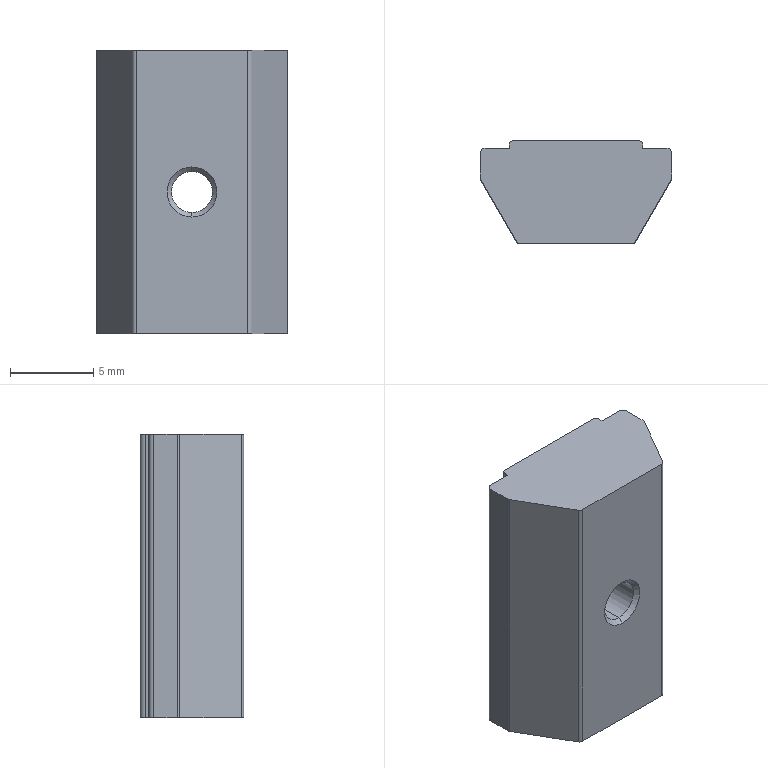Part | SolidWorks | features BaseBody 1 | 1 solid | 26 faces | box 11.5 x 6.2 x 17 mm | volume 1002 mm3 | plane 12 | cylinder 10 | cone 4 | commonest cylinder face diameters 0.6 x8 2.459 x2
STEP:
#1=CARTESIAN_POINT('',(0.,5.93,-9.729));
#2=VERTEX_POINT('',#1);
#3=CARTESIAN_POINT('',(0.,5.93,-7.271));
#4=VERTEX_POINT('',#3);
#5=CARTESIAN_POINT('',(0.,5.93,-8.5));
#6=DIRECTION('',(0.,1.,0.));
#7=DIRECTION('',(0.,0.,1.));
#8=AXIS2_PLACEMENT_3D('',#5,#6,#7);
#9=CIRCLE('',#8,1.229);
#10=EDGE_CURVE('',#2,#4,#9,.T.);
#11=ORIENTED_EDGE('',*,*,#10,.F.);
#12=CARTESIAN_POINT('',(0.,6.2,-10.));
#13=VERTEX_POINT('',#12);
#14=CARTESIAN_POINT('',(0.,6.2,-10.));
#15=DIRECTION('',(0.,0.7071,-0.7071));
#16=VECTOR('',#15,1000.);
#17=LINE('',#14,#16);
#18=EDGE_CURVE('',#2,#13,#17,.T.);
#19=ORIENTED_EDGE('',*,*,#18,.T.);
#20=CARTESIAN_POINT('',(0.,6.2,-7.));
#21=VERTEX_POINT('',#20);
#22=CARTESIAN_POINT('',(0.,6.2,-8.5));
#23=DIRECTION('',(0.,-1.,0.));
#24=DIRECTION('',(0.,0.,1.));
#25=AXIS2_PLACEMENT_3D('',#22,#23,#24);
#26=CIRCLE('',#25,1.5);
#27=EDGE_CURVE('',#21,#13,#26,.T.);
#28=ORIENTED_EDGE('',*,*,#27,.F.);
#29=CARTESIAN_POINT('',(0.,6.2,-7.));
#30=DIRECTION('',(0.,0.7071,0.7071));
#31=VECTOR('',#30,1000.);
#32=LINE('',#29,#31);
#33=EDGE_CURVE('',#4,#21,#32,.T.);
#34=ORIENTED_EDGE('',*,*,#33,.F.);
#35=EDGE_LOOP('',(#11,#19,#28,#34));
#36=FACE_OUTER_BOUND('',#35,.T.);
#37=CARTESIAN_POINT('',(0.,6.2,-8.5));
#38=DIRECTION('',(0.,1.,0.));
#39=DIRECTION('',(0.,0.,1.));
#40=AXIS2_PLACEMENT_3D('',#37,#38,#39);
#41=CONICAL_SURFACE('',#40,1.5,0.7854);
#42=ADVANCED_FACE('',(#36),#41,.F.);
#43=CARTESIAN_POINT('',(0.,0.2705,-9.729));
#44=VERTEX_POINT('',#43);
#45=CARTESIAN_POINT('',(0.,0.2705,-7.271));
#46=VERTEX_POINT('',#45);
#47=CARTESIAN_POINT('',(0.,0.2705,-8.5));
#48=DIRECTION('',(0.,1.,0.));
#49=DIRECTION('',(0.,0.,1.));
#50=AXIS2_PLACEMENT_3D('',#47,#48,#49);
#51=CIRCLE('',#50,1.229);
#52=EDGE_CURVE('',#44,#46,#51,.T.);
#53=ORIENTED_EDGE('',*,*,#52,.F.);
#54=CARTESIAN_POINT('',(0.,0.,-9.729));
#55=DIRECTION('',(0.,1.,0.));
#56=VECTOR('',#55,1000.);
#57=LINE('',#54,#56);
#58=EDGE_CURVE('',#44,#2,#57,.T.);
#59=ORIENTED_EDGE('',*,*,#58,.T.);
#60=ORIENTED_EDGE('',*,*,#10,.T.);
#61=CARTESIAN_POINT('',(0.,0.,-7.271));
#62=DIRECTION('',(0.,1.,0.));
#63=VECTOR('',#62,1000.);
#64=LINE('',#61,#63);
#65=EDGE_CURVE('',#46,#4,#64,.T.);
#66=ORIENTED_EDGE('',*,*,#65,.F.);
#67=EDGE_LOOP('',(#53,#59,#60,#66));
#68=FACE_OUTER_BOUND('',#67,.T.);
#69=CARTESIAN_POINT('',(0.,0.,-8.5));
#70=DIRECTION('',(0.,1.,0.));
#71=DIRECTION('',(0.,0.,1.));
#72=AXIS2_PLACEMENT_3D('',#69,#70,#71);
#73=CYLINDRICAL_SURFACE('',#72,1.229);
#74=ADVANCED_FACE('',(#68),#73,.F.);
#75=ORIENTED_EDGE('',*,*,#52,.T.);
#76=CARTESIAN_POINT('',(0.,0.,-7.));
#77=VERTEX_POINT('',#76);
#78=CARTESIAN_POINT('',(0.,0.,-7.));
#79=DIRECTION('',(0.,-0.7071,0.7071));
#80=VECTOR('',#79,1000.);
#81=LINE('',#78,#80);
#82=EDGE_CURVE('',#46,#77,#81,.T.);
#83=ORIENTED_EDGE('',*,*,#82,.T.);
#84=CARTESIAN_POINT('',(0.,0.,-10.));
#85=VERTEX_POINT('',#84);
#86=CARTESIAN_POINT('',(0.,0.,-8.5));
#87=DIRECTION('',(0.,1.,0.));
#88=DIRECTION('',(0.,0.,-1.));
#89=AXIS2_PLACEMENT_3D('',#86,#87,#88);
#90=CIRCLE('',#89,1.5);
#91=EDGE_CURVE('',#85,#77,#90,.T.);
#92=ORIENTED_EDGE('',*,*,#91,.F.);
#93=CARTESIAN_POINT('',(0.,0.,-10.));
#94=DIRECTION('',(0.,-0.7071,-0.7071));
#95=VECTOR('',#94,1000.);
#96=LINE('',#93,#95);
#97=EDGE_CURVE('',#44,#85,#96,.T.);
#98=ORIENTED_EDGE('',*,*,#97,.F.);
#99=EDGE_LOOP('',(#75,#83,#92,#98));
#100=FACE_OUTER_BOUND('',#99,.T.);
#101=CARTESIAN_POINT('',(0.,0.,-8.5));
#102=DIRECTION('',(0.,-1.,0.));
#103=DIRECTION('',(0.,0.,-1.));
#104=AXIS2_PLACEMENT_3D('',#101,#102,#103);
#105=CONICAL_SURFACE('',#104,1.5,0.7854);
#106=ADVANCED_FACE('',(#100),#105,.F.);
#107=CARTESIAN_POINT('',(3.7,6.2,-17.));
#108=VERTEX_POINT('',#107);
#109=CARTESIAN_POINT('',(-3.7,6.2,-17.));
#110=VERTEX_POINT('',#109);
#111=CARTESIAN_POINT('',(3.7,6.2,-17.));
#112=DIRECTION('',(-1.,0.,0.));
#113=VECTOR('',#112,1000.);
#114=LINE('',#111,#113);
#115=EDGE_CURVE('',#108,#110,#114,.T.);
#116=ORIENTED_EDGE('',*,*,#115,.T.);
#117=CARTESIAN_POINT('',(-3.7,6.2,0.));
#118=VERTEX_POINT('',#117);
#119=CARTESIAN_POINT('',(-3.7,6.2,-17.));
#120=DIRECTION('',(0.,0.,1.));
#121=VECTOR('',#120,1000.);
#122=LINE('',#119,#121);
#123=EDGE_CURVE('',#110,#118,#122,.T.);
#124=ORIENTED_EDGE('',*,*,#123,.T.);
#125=CARTESIAN_POINT('',(3.7,6.2,0.));
#126=VERTEX_POINT('',#125);
#127=CARTESIAN_POINT('',(3.7,6.2,0.));
#128=DIRECTION('',(1.,0.,0.));
#129=VECTOR('',#128,1000.);
#130=LINE('',#127,#129);
#131=EDGE_CURVE('',#118,#126,#130,.T.);
#132=ORIENTED_EDGE('',*,*,#131,.T.);
#133=CARTESIAN_POINT('',(3.7,6.2,-17.));
#134=DIRECTION('',(0.,0.,-1.));
#135=VECTOR('',#134,1000.);
#136=LINE('',#133,#135);
#137=EDGE_CURVE('',#126,#108,#136,.T.);
#138=ORIENTED_EDGE('',*,*,#137,.T.);
#139=EDGE_LOOP('',(#116,#124,#132,#138));
#140=FACE_OUTER_BOUND('',#139,.T.);
#141=ORIENTED_EDGE('',*,*,#27,.T.);
#142=CARTESIAN_POINT('',(0.,6.2,-8.5));
#143=DIRECTION('',(0.,-1.,0.));
#144=DIRECTION('',(0.,0.,1.));
#145=AXIS2_PLACEMENT_3D('',#142,#143,#144);
#146=CIRCLE('',#145,1.5);
#147=EDGE_CURVE('',#13,#21,#146,.T.);
#148=ORIENTED_EDGE('',*,*,#147,.T.);
#149=EDGE_LOOP('',(#141,#148));
#150=FACE_BOUND('',#149,.T.);
#151=CARTESIAN_POINT('',(3.7,6.2,-17.));
#152=DIRECTION('',(0.,1.,0.));
#153=DIRECTION('',(0.,0.,1.));
#154=AXIS2_PLACEMENT_3D('',#151,#152,#153);
#155=PLANE('',#154);
#156=ADVANCED_FACE('',(#140,#150),#155,.T.);
#157=CARTESIAN_POINT('',(-4.,5.9,-17.));
#158=VERTEX_POINT('',#157);
#159=CARTESIAN_POINT('',(-3.7,5.9,-17.));
#160=DIRECTION('',(0.,0.,1.));
#161=DIRECTION('',(-1.,0.,0.));
#162=AXIS2_PLACEMENT_3D('',#159,#160,#161);
#163=CIRCLE('',#162,0.3);
#164=EDGE_CURVE('',#110,#158,#163,.T.);
#165=ORIENTED_EDGE('',*,*,#164,.T.);
#166=CARTESIAN_POINT('',(-4.,5.9,0.));
#167=VERTEX_POINT('',#166);
#168=CARTESIAN_POINT('',(-4.,5.9,-17.));
#169=DIRECTION('',(0.,0.,1.));
#170=VECTOR('',#169,1000.);
#171=LINE('',#168,#170);
#172=EDGE_CURVE('',#158,#167,#171,.T.);
#173=ORIENTED_EDGE('',*,*,#172,.T.);
#174=CARTESIAN_POINT('',(-3.7,5.9,0.));
#175=DIRECTION('',(0.,0.,-1.));
#176=DIRECTION('',(-1.,0.,0.));
#177=AXIS2_PLACEMENT_3D('',#174,#175,#176);
#178=CIRCLE('',#177,0.3);
#179=EDGE_CURVE('',#167,#118,#178,.T.);
#180=ORIENTED_EDGE('',*,*,#179,.T.);
#181=ORIENTED_EDGE('',*,*,#123,.F.);
#182=EDGE_LOOP('',(#165,#173,#180,#181));
#183=FACE_OUTER_BOUND('',#182,.T.);
#184=CARTESIAN_POINT('',(-3.7,5.9,-17.));
#185=DIRECTION('',(0.,0.,-1.));
#186=DIRECTION('',(-1.,0.,0.));
#187=AXIS2_PLACEMENT_3D('',#184,#185,#186);
#188=CYLINDRICAL_SURFACE('',#187,0.3);
#189=ADVANCED_FACE('',(#183),#188,.T.);
#190=CARTESIAN_POINT('',(-4.,5.7,-17.));
#191=VERTEX_POINT('',#190);
#192=CARTESIAN_POINT('',(-5.45,5.7,-17.));
#193=VERTEX_POINT('',#192);
#194=CARTESIAN_POINT('',(-4.,5.7,-17.));
#195=DIRECTION('',(-1.,0.,0.));
#196=VECTOR('',#195,1000.);
#197=LINE('',#194,#196);
#198=EDGE_CURVE('',#191,#193,#197,.T.);
#199=ORIENTED_EDGE('',*,*,#198,.F.);
#200=CARTESIAN_POINT('',(-4.,5.4,-17.));
#201=DIRECTION('',(0.,-1.,0.));
#202=VECTOR('',#201,1000.);
#203=LINE('',#200,#202);
#204=EDGE_CURVE('',#158,#191,#203,.T.);
#205=ORIENTED_EDGE('',*,*,#204,.F.);
#206=ORIENTED_EDGE('',*,*,#164,.F.);
#207=ORIENTED_EDGE('',*,*,#115,.F.);
#208=CARTESIAN_POINT('',(4.,5.9,-17.));
#209=VERTEX_POINT('',#208);
#210=CARTESIAN_POINT('',(3.7,5.9,-17.));
#211=DIRECTION('',(0.,0.,1.));
#212=DIRECTION('',(-1.,0.,0.));
#213=AXIS2_PLACEMENT_3D('',#210,#211,#212);
#214=CIRCLE('',#213,0.3);
#215=EDGE_CURVE('',#209,#108,#214,.T.);
#216=ORIENTED_EDGE('',*,*,#215,.F.);
#217=CARTESIAN_POINT('',(4.,5.7,-17.));
#218=VERTEX_POINT('',#217);
#219=CARTESIAN_POINT('',(4.,5.7,-17.));
#220=DIRECTION('',(0.,1.,0.));
#221=VECTOR('',#220,1000.);
#222=LINE('',#219,#221);
#223=EDGE_CURVE('',#218,#209,#222,.T.);
#224=ORIENTED_EDGE('',*,*,#223,.F.);
#225=CARTESIAN_POINT('',(5.45,5.7,-17.));
#226=VERTEX_POINT('',#225);
#227=CARTESIAN_POINT('',(5.45,5.7,-17.));
#228=DIRECTION('',(-1.,0.,0.));
#229=VECTOR('',#228,1000.);
#230=LINE('',#227,#229);
#231=EDGE_CURVE('',#226,#218,#230,.T.);
#232=ORIENTED_EDGE('',*,*,#231,.F.);
#233=CARTESIAN_POINT('',(5.75,5.4,-17.));
#234=VERTEX_POINT('',#233);
#235=CARTESIAN_POINT('',(5.45,5.4,-17.));
#236=DIRECTION('',(0.,0.,1.));
#237=DIRECTION('',(-1.,0.,0.));
#238=AXIS2_PLACEMENT_3D('',#235,#236,#237);
#239=CIRCLE('',#238,0.3);
#240=EDGE_CURVE('',#234,#226,#239,.T.);
#241=ORIENTED_EDGE('',*,*,#240,.F.);
#242=CARTESIAN_POINT('',(5.75,3.978,-17.));
#243=VERTEX_POINT('',#242);
#244=CARTESIAN_POINT('',(5.75,3.978,-17.));
#245=DIRECTION('',(0.,1.,0.));
#246=VECTOR('',#245,1000.);
#247=LINE('',#244,#246);
#248=EDGE_CURVE('',#243,#234,#247,.T.);
#249=ORIENTED_EDGE('',*,*,#248,.F.);
#250=CARTESIAN_POINT('',(5.71,3.828,-17.));
#251=VERTEX_POINT('',#250);
#252=CARTESIAN_POINT('',(5.45,3.978,-17.));
#253=DIRECTION('',(0.,0.,1.));
#254=DIRECTION('',(-1.,0.,0.));
#255=AXIS2_PLACEMENT_3D('',#252,#253,#254);
#256=CIRCLE('',#255,0.3);
#257=EDGE_CURVE('',#251,#243,#256,.T.);
#258=ORIENTED_EDGE('',*,*,#257,.F.);
#259=CARTESIAN_POINT('',(3.586,0.15,-17.));
#260=VERTEX_POINT('',#259);
#261=CARTESIAN_POINT('',(3.586,0.15,-17.));
#262=DIRECTION('',(0.5001,0.866,0.));
#263=VECTOR('',#262,1000.);
#264=LINE('',#261,#263);
#265=EDGE_CURVE('',#260,#251,#264,.T.);
#266=ORIENTED_EDGE('',*,*,#265,.F.);
#267=CARTESIAN_POINT('',(3.326,0.,-17.));
#268=VERTEX_POINT('',#267);
#269=CARTESIAN_POINT('',(3.326,0.3,-17.));
#270=DIRECTION('',(0.,0.,1.));
#271=DIRECTION('',(-1.,0.,0.));
#272=AXIS2_PLACEMENT_3D('',#269,#270,#271);
#273=CIRCLE('',#272,0.3);
#274=EDGE_CURVE('',#268,#260,#273,.T.);
#275=ORIENTED_EDGE('',*,*,#274,.F.);
#276=CARTESIAN_POINT('',(-3.327,0.,-17.));
#277=VERTEX_POINT('',#276);
#278=CARTESIAN_POINT('',(-5.45,0.,-17.));
#279=DIRECTION('',(1.,0.,0.));
#280=VECTOR('',#279,1000.);
#281=LINE('',#278,#280);
#282=EDGE_CURVE('',#277,#268,#281,.T.);
#283=ORIENTED_EDGE('',*,*,#282,.F.);
#284=CARTESIAN_POINT('',(-3.587,0.15,-17.));
#285=VERTEX_POINT('',#284);
#286=CARTESIAN_POINT('',(-3.327,0.3,-17.));
#287=DIRECTION('',(0.,0.,1.));
#288=DIRECTION('',(-1.,0.,0.));
#289=AXIS2_PLACEMENT_3D('',#286,#287,#288);
#290=CIRCLE('',#289,0.3);
#291=EDGE_CURVE('',#285,#277,#290,.T.);
#292=ORIENTED_EDGE('',*,*,#291,.F.);
#293=CARTESIAN_POINT('',(-5.71,3.828,-17.));
#294=VERTEX_POINT('',#293);
#295=CARTESIAN_POINT('',(-5.71,3.828,-17.));
#296=DIRECTION('',(0.4999,-0.8661,0.));
#297=VECTOR('',#296,1000.);
#298=LINE('',#295,#297);
#299=EDGE_CURVE('',#294,#285,#298,.T.);
#300=ORIENTED_EDGE('',*,*,#299,.F.);
#301=CARTESIAN_POINT('',(-5.75,3.978,-17.));
#302=VERTEX_POINT('',#301);
#303=CARTESIAN_POINT('',(-5.45,3.978,-17.));
#304=DIRECTION('',(0.,0.,1.));
#305=DIRECTION('',(-1.,0.,0.));
#306=AXIS2_PLACEMENT_3D('',#303,#304,#305);
#307=CIRCLE('',#306,0.3);
#308=EDGE_CURVE('',#302,#294,#307,.T.);
#309=ORIENTED_EDGE('',*,*,#308,.F.);
#310=CARTESIAN_POINT('',(-5.75,5.4,-17.));
#311=VERTEX_POINT('',#310);
#312=CARTESIAN_POINT('',(-5.75,5.4,-17.));
#313=DIRECTION('',(0.,-1.,0.));
#314=VECTOR('',#313,1000.);
#315=LINE('',#312,#314);
#316=EDGE_CURVE('',#311,#302,#315,.T.);
#317=ORIENTED_EDGE('',*,*,#316,.F.);
#318=CARTESIAN_POINT('',(-5.45,5.4,-17.));
#319=DIRECTION('',(0.,0.,1.));
#320=DIRECTION('',(-1.,0.,0.));
#321=AXIS2_PLACEMENT_3D('',#318,#319,#320);
#322=CIRCLE('',#321,0.3);
#323=EDGE_CURVE('',#193,#311,#322,.T.);
#324=ORIENTED_EDGE('',*,*,#323,.F.);
#325=EDGE_LOOP('',(#199,#205,#206,#207,#216,#224,#232,#241,#249,#258,#266,#275,#283,#292,#300,#309,#317,#324));
#326=FACE_OUTER_BOUND('',#325,.T.);
#327=CARTESIAN_POINT('',(-5.45,5.4,-17.));
#328=DIRECTION('',(0.,0.,1.));
#329=DIRECTION('',(1.,0.,0.));
#330=AXIS2_PLACEMENT_3D('',#327,#328,#329);
#331=PLANE('',#330);
#332=ADVANCED_FACE('',(#326),#331,.F.);
#333=ORIENTED_EDGE('',*,*,#215,.T.);
#334=ORIENTED_EDGE('',*,*,#137,.F.);
#335=CARTESIAN_POINT('',(4.,5.9,0.));
#336=VERTEX_POINT('',#335);
#337=CARTESIAN_POINT('',(3.7,5.9,0.));
#338=DIRECTION('',(0.,0.,-1.));
#339=DIRECTION('',(-1.,0.,0.));
#340=AXIS2_PLACEMENT_3D('',#337,#338,#339);
#341=CIRCLE('',#340,0.3);
#342=EDGE_CURVE('',#126,#336,#341,.T.);
#343=ORIENTED_EDGE('',*,*,#342,.T.);
#344=CARTESIAN_POINT('',(4.,5.9,-17.));
#345=DIRECTION('',(0.,0.,-1.));
#346=VECTOR('',#345,1000.);
#347=LINE('',#344,#346);
#348=EDGE_CURVE('',#336,#209,#347,.T.);
#349=ORIENTED_EDGE('',*,*,#348,.T.);
#350=EDGE_LOOP('',(#333,#334,#343,#349));
#351=FACE_OUTER_BOUND('',#350,.T.);
#352=CARTESIAN_POINT('',(3.7,5.9,-17.));
#353=DIRECTION('',(0.,0.,-1.));
#354=DIRECTION('',(-1.,0.,0.));
#355=AXIS2_PLACEMENT_3D('',#352,#353,#354);
#356=CYLINDRICAL_SURFACE('',#355,0.3);
#357=ADVANCED_FACE('',(#351),#356,.T.);
#358=CARTESIAN_POINT('',(-4.,5.7,0.));
#359=VERTEX_POINT('',#358);
#360=CARTESIAN_POINT('',(-4.,5.4,0.));
#361=DIRECTION('',(0.,-1.,0.));
#362=VECTOR('',#361,1000.);
#363=LINE('',#360,#362);
#364=EDGE_CURVE('',#167,#359,#363,.T.);
#365=ORIENTED_EDGE('',*,*,#364,.T.);
#366=CARTESIAN_POINT('',(-5.45,5.7,0.));
#367=VERTEX_POINT('',#366);
#368=CARTESIAN_POINT('',(-4.,5.7,0.));
#369=DIRECTION('',(1.,0.,0.));
#370=VECTOR('',#369,1000.);
#371=LINE('',#368,#370);
#372=EDGE_CURVE('',#367,#359,#371,.T.);
#373=ORIENTED_EDGE('',*,*,#372,.F.);
#374=CARTESIAN_POINT('',(-5.75,5.4,0.));
#375=VERTEX_POINT('',#374);
#376=CARTESIAN_POINT('',(-5.45,5.4,0.));
#377=DIRECTION('',(0.,0.,-1.));
#378=DIRECTION('',(-1.,0.,0.));
#379=AXIS2_PLACEMENT_3D('',#376,#377,#378);
#380=CIRCLE('',#379,0.3);
#381=EDGE_CURVE('',#375,#367,#380,.T.);
#382=ORIENTED_EDGE('',*,*,#381,.F.);
#383=CARTESIAN_POINT('',(-5.75,3.978,0.));
#384=VERTEX_POINT('',#383);
#385=CARTESIAN_POINT('',(-5.75,5.4,0.));
#386=DIRECTION('',(0.,1.,0.));
#387=VECTOR('',#386,1000.);
#388=LINE('',#385,#387);
#389=EDGE_CURVE('',#384,#375,#388,.T.);
#390=ORIENTED_EDGE('',*,*,#389,.F.);
#391=CARTESIAN_POINT('',(-5.71,3.828,0.));
#392=VERTEX_POINT('',#391);
#393=CARTESIAN_POINT('',(-5.45,3.978,0.));
#394=DIRECTION('',(0.,0.,-1.));
#395=DIRECTION('',(-1.,0.,0.));
#396=AXIS2_PLACEMENT_3D('',#393,#394,#395);
#397=CIRCLE('',#396,0.3);
#398=EDGE_CURVE('',#392,#384,#397,.T.);
#399=ORIENTED_EDGE('',*,*,#398,.F.);
#400=CARTESIAN_POINT('',(-3.587,0.15,0.));
#401=VERTEX_POINT('',#400);
#402=CARTESIAN_POINT('',(-5.71,3.828,0.));
#403=DIRECTION('',(0.4999,-0.8661,0.));
#404=VECTOR('',#403,1000.);
#405=LINE('',#402,#404);
#406=EDGE_CURVE('',#392,#401,#405,.T.);
#407=ORIENTED_EDGE('',*,*,#406,.T.);
#408=CARTESIAN_POINT('',(-3.327,0.,0.));
#409=VERTEX_POINT('',#408);
#410=CARTESIAN_POINT('',(-3.327,0.3,0.));
#411=DIRECTION('',(0.,0.,-1.));
#412=DIRECTION('',(-1.,0.,0.));
#413=AXIS2_PLACEMENT_3D('',#410,#411,#412);
#414=CIRCLE('',#413,0.3);
#415=EDGE_CURVE('',#409,#401,#414,.T.);
#416=ORIENTED_EDGE('',*,*,#415,.F.);
#417=CARTESIAN_POINT('',(3.326,0.,0.));
#418=VERTEX_POINT('',#417);
#419=CARTESIAN_POINT('',(-5.45,0.,0.));
#420=DIRECTION('',(1.,0.,0.));
#421=VECTOR('',#420,1000.);
#422=LINE('',#419,#421);
#423=EDGE_CURVE('',#409,#418,#422,.T.);
#424=ORIENTED_EDGE('',*,*,#423,.T.);
#425=CARTESIAN_POINT('',(3.586,0.15,0.));
#426=VERTEX_POINT('',#425);
#427=CARTESIAN_POINT('',(3.326,0.3,0.));
#428=DIRECTION('',(0.,0.,-1.));
#429=DIRECTION('',(-1.,0.,0.));
#430=AXIS2_PLACEMENT_3D('',#427,#428,#429);
#431=CIRCLE('',#430,0.3);
#432=EDGE_CURVE('',#426,#418,#431,.T.);
#433=ORIENTED_EDGE('',*,*,#432,.F.);
#434=CARTESIAN_POINT('',(5.71,3.828,0.));
#435=VERTEX_POINT('',#434);
#436=CARTESIAN_POINT('',(3.586,0.15,0.));
#437=DIRECTION('',(0.5001,0.866,0.));
#438=VECTOR('',#437,1000.);
#439=LINE('',#436,#438);
#440=EDGE_CURVE('',#426,#435,#439,.T.);
#441=ORIENTED_EDGE('',*,*,#440,.T.);
#442=CARTESIAN_POINT('',(5.75,3.978,0.));
#443=VERTEX_POINT('',#442);
#444=CARTESIAN_POINT('',(5.45,3.978,0.));
#445=DIRECTION('',(0.,0.,-1.));
#446=DIRECTION('',(-1.,0.,0.));
#447=AXIS2_PLACEMENT_3D('',#444,#445,#446);
#448=CIRCLE('',#447,0.3);
#449=EDGE_CURVE('',#443,#435,#448,.T.);
#450=ORIENTED_EDGE('',*,*,#449,.F.);
#451=CARTESIAN_POINT('',(5.75,5.4,0.));
#452=VERTEX_POINT('',#451);
#453=CARTESIAN_POINT('',(5.75,3.978,0.));
#454=DIRECTION('',(0.,-1.,0.));
#455=VECTOR('',#454,1000.);
#456=LINE('',#453,#455);
#457=EDGE_CURVE('',#452,#443,#456,.T.);
#458=ORIENTED_EDGE('',*,*,#457,.F.);
#459=CARTESIAN_POINT('',(5.45,5.7,0.));
#460=VERTEX_POINT('',#459);
#461=CARTESIAN_POINT('',(5.45,5.4,0.));
#462=DIRECTION('',(0.,0.,-1.));
#463=DIRECTION('',(-1.,0.,0.));
#464=AXIS2_PLACEMENT_3D('',#461,#462,#463);
#465=CIRCLE('',#464,0.3);
#466=EDGE_CURVE('',#460,#452,#465,.T.);
#467=ORIENTED_EDGE('',*,*,#466,.F.);
#468=CARTESIAN_POINT('',(4.,5.7,0.));
#469=VERTEX_POINT('',#468);
#470=CARTESIAN_POINT('',(5.45,5.7,0.));
#471=DIRECTION('',(1.,0.,0.));
#472=VECTOR('',#471,1000.);
#473=LINE('',#470,#472);
#474=EDGE_CURVE('',#469,#460,#473,.T.);
#475=ORIENTED_EDGE('',*,*,#474,.F.);
#476=CARTESIAN_POINT('',(4.,5.4,0.));
#477=DIRECTION('',(0.,1.,0.));
#478=VECTOR('',#477,1000.);
#479=LINE('',#476,#478);
#480=EDGE_CURVE('',#469,#336,#479,.T.);
#481=ORIENTED_EDGE('',*,*,#480,.T.);
#482=ORIENTED_EDGE('',*,*,#342,.F.);
#483=ORIENTED_EDGE('',*,*,#131,.F.);
#484=ORIENTED_EDGE('',*,*,#179,.F.);
#485=EDGE_LOOP('',(#365,#373,#382,#390,#399,#407,#416,#424,#433,#441,#450,#458,#467,#475,#481,#482,#483,#484));
#486=FACE_OUTER_BOUND('',#485,.T.);
#487=CARTESIAN_POINT('',(-5.45,5.4,0.));
#488=DIRECTION('',(0.,0.,1.));
#489=DIRECTION('',(1.,0.,0.));
#490=AXIS2_PLACEMENT_3D('',#487,#488,#489);
#491=PLANE('',#490);
#492=ADVANCED_FACE('',(#486),#491,.T.);
#493=ORIENTED_EDGE('',*,*,#18,.F.);
#494=CARTESIAN_POINT('',(0.,5.93,-8.5));
#495=DIRECTION('',(0.,1.,0.));
#496=DIRECTION('',(0.,0.,1.));
#497=AXIS2_PLACEMENT_3D('',#494,#495,#496);
#498=CIRCLE('',#497,1.229);
#499=EDGE_CURVE('',#4,#2,#498,.T.);
#500=ORIENTED_EDGE('',*,*,#499,.F.);
#501=ORIENTED_EDGE('',*,*,#33,.T.);
#502=ORIENTED_EDGE('',*,*,#147,.F.);
#503=EDGE_LOOP('',(#493,#500,#501,#502));
#504=FACE_OUTER_BOUND('',#503,.T.);
#505=CARTESIAN_POINT('',(0.,6.2,-8.5));
#506=DIRECTION('',(0.,1.,0.));
#507=DIRECTION('',(0.,0.,1.));
#508=AXIS2_PLACEMENT_3D('',#505,#506,#507);
#509=CONICAL_SURFACE('',#508,1.5,0.7854);
#510=ADVANCED_FACE('',(#504),#509,.F.);
#511=ORIENTED_EDGE('',*,*,#204,.T.);
#512=CARTESIAN_POINT('',(-4.,5.7,-17.));
#513=DIRECTION('',(0.,0.,1.));
#514=VECTOR('',#513,1000.);
#515=LINE('',#512,#514);
#516=EDGE_CURVE('',#191,#359,#515,.T.);
#517=ORIENTED_EDGE('',*,*,#516,.T.);
#518=ORIENTED_EDGE('',*,*,#364,.F.);
#519=ORIENTED_EDGE('',*,*,#172,.F.);
#520=EDGE_LOOP('',(#511,#517,#518,#519));
#521=FACE_OUTER_BOUND('',#520,.T.);
#522=CARTESIAN_POINT('',(-4.,5.9,-17.));
#523=DIRECTION('',(-1.,0.,0.));
#524=DIRECTION('',(0.,0.,1.));
#525=AXIS2_PLACEMENT_3D('',#522,#523,#524);
#526=PLANE('',#525);
#527=ADVANCED_FACE('',(#521),#526,.T.);
#528=ORIENTED_EDGE('',*,*,#265,.T.);
#529=CARTESIAN_POINT('',(5.71,3.828,-17.));
#530=DIRECTION('',(0.,0.,1.));
#531=VECTOR('',#530,1000.);
#532=LINE('',#529,#531);
#533=EDGE_CURVE('',#251,#435,#532,.T.);
#534=ORIENTED_EDGE('',*,*,#533,.T.);
#535=ORIENTED_EDGE('',*,*,#440,.F.);
#536=CARTESIAN_POINT('',(3.586,0.15,-17.));
#537=DIRECTION('',(0.,0.,-1.));
#538=VECTOR('',#537,1000.);
#539=LINE('',#536,#538);
#540=EDGE_CURVE('',#426,#260,#539,.T.);
#541=ORIENTED_EDGE('',*,*,#540,.T.);
#542=EDGE_LOOP('',(#528,#534,#535,#541));
#543=FACE_OUTER_BOUND('',#542,.T.);
#544=CARTESIAN_POINT('',(3.586,0.15,-17.));
#545=DIRECTION('',(0.866,-0.5001,0.));
#546=DIRECTION('',(0.5001,0.866,0.));
#547=AXIS2_PLACEMENT_3D('',#544,#545,#546);
#548=PLANE('',#547);
#549=ADVANCED_FACE('',(#543),#548,.T.);
#550=ORIENTED_EDGE('',*,*,#282,.T.);
#551=CARTESIAN_POINT('',(3.326,0.,-17.));
#552=DIRECTION('',(0.,0.,1.));
#553=VECTOR('',#552,1000.);
#554=LINE('',#551,#553);
#555=EDGE_CURVE('',#268,#418,#554,.T.);
#556=ORIENTED_EDGE('',*,*,#555,.T.);
#557=ORIENTED_EDGE('',*,*,#423,.F.);
#558=CARTESIAN_POINT('',(-3.327,0.,-17.));
#559=DIRECTION('',(0.,0.,-1.));
#560=VECTOR('',#559,1000.);
#561=LINE('',#558,#560);
#562=EDGE_CURVE('',#409,#277,#561,.T.);
#563=ORIENTED_EDGE('',*,*,#562,.T.);
#564=EDGE_LOOP('',(#550,#556,#557,#563));
#565=FACE_OUTER_BOUND('',#564,.T.);
#566=ORIENTED_EDGE('',*,*,#91,.T.);
#567=CARTESIAN_POINT('',(0.,0.,-8.5));
#568=DIRECTION('',(0.,1.,0.));
#569=DIRECTION('',(0.,0.,-1.));
#570=AXIS2_PLACEMENT_3D('',#567,#568,#569);
#571=CIRCLE('',#570,1.5);
#572=EDGE_CURVE('',#77,#85,#571,.T.);
#573=ORIENTED_EDGE('',*,*,#572,.T.);
#574=EDGE_LOOP('',(#566,#573));
#575=FACE_BOUND('',#574,.T.);
#576=CARTESIAN_POINT('',(-3.327,0.,-17.));
#577=DIRECTION('',(0.,-1.,0.));
#578=DIRECTION('',(0.,0.,-1.));
#579=AXIS2_PLACEMENT_3D('',#576,#577,#578);
#580=PLANE('',#579);
#581=ADVANCED_FACE('',(#565,#575),#580,.T.);
#582=ORIENTED_EDGE('',*,*,#299,.T.);
#583=CARTESIAN_POINT('',(-3.587,0.15,-17.));
#584=DIRECTION('',(0.,0.,1.));
#585=VECTOR('',#584,1000.);
#586=LINE('',#583,#585);
#587=EDGE_CURVE('',#285,#401,#586,.T.);
#588=ORIENTED_EDGE('',*,*,#587,.T.);
#589=ORIENTED_EDGE('',*,*,#406,.F.);
#590=CARTESIAN_POINT('',(-5.71,3.828,-17.));
#591=DIRECTION('',(0.,0.,-1.));
#592=VECTOR('',#591,1000.);
#593=LINE('',#590,#592);
#594=EDGE_CURVE('',#392,#294,#593,.T.);
#595=ORIENTED_EDGE('',*,*,#594,.T.);
#596=EDGE_LOOP('',(#582,#588,#589,#595));
#597=FACE_OUTER_BOUND('',#596,.T.);
#598=CARTESIAN_POINT('',(-5.71,3.828,-17.));
#599=DIRECTION('',(-0.8661,-0.4999,0.));
#600=DIRECTION('',(0.4999,-0.8661,0.));
#601=AXIS2_PLACEMENT_3D('',#598,#599,#600);
#602=PLANE('',#601);
#603=ADVANCED_FACE('',(#597),#602,.T.);
#604=ORIENTED_EDGE('',*,*,#223,.T.);
#605=ORIENTED_EDGE('',*,*,#348,.F.);
#606=ORIENTED_EDGE('',*,*,#480,.F.);
#607=CARTESIAN_POINT('',(4.,5.7,-17.));
#608=DIRECTION('',(0.,0.,-1.));
#609=VECTOR('',#608,1000.);
#610=LINE('',#607,#609);
#611=EDGE_CURVE('',#469,#218,#610,.T.);
#612=ORIENTED_EDGE('',*,*,#611,.T.);
#613=EDGE_LOOP('',(#604,#605,#606,#612));
#614=FACE_OUTER_BOUND('',#613,.T.);
#615=CARTESIAN_POINT('',(4.,5.7,-17.));
#616=DIRECTION('',(1.,0.,0.));
#617=DIRECTION('',(0.,0.,-1.));
#618=AXIS2_PLACEMENT_3D('',#615,#616,#617);
#619=PLANE('',#618);
#620=ADVANCED_FACE('',(#614),#619,.T.);
#621=ORIENTED_EDGE('',*,*,#58,.F.);
#622=CARTESIAN_POINT('',(0.,0.2705,-8.5));
#623=DIRECTION('',(0.,1.,0.));
#624=DIRECTION('',(0.,0.,1.));
#625=AXIS2_PLACEMENT_3D('',#622,#623,#624);
#626=CIRCLE('',#625,1.229);
#627=EDGE_CURVE('',#46,#44,#626,.T.);
#628=ORIENTED_EDGE('',*,*,#627,.F.);
#629=ORIENTED_EDGE('',*,*,#65,.T.);
#630=ORIENTED_EDGE('',*,*,#499,.T.);
#631=EDGE_LOOP('',(#621,#628,#629,#630));
#632=FACE_OUTER_BOUND('',#631,.T.);
#633=CARTESIAN_POINT('',(0.,0.,-8.5));
#634=DIRECTION('',(0.,1.,0.));
#635=DIRECTION('',(0.,0.,1.));
#636=AXIS2_PLACEMENT_3D('',#633,#634,#635);
#637=CYLINDRICAL_SURFACE('',#636,1.229);
#638=ADVANCED_FACE('',(#632),#637,.F.);
#639=ORIENTED_EDGE('',*,*,#198,.T.);
#640=CARTESIAN_POINT('',(-5.45,5.7,-17.));
#641=DIRECTION('',(0.,0.,1.));
#642=VECTOR('',#641,1000.);
#643=LINE('',#640,#642);
#644=EDGE_CURVE('',#193,#367,#643,.T.);
#645=ORIENTED_EDGE('',*,*,#644,.T.);
#646=ORIENTED_EDGE('',*,*,#372,.T.);
#647=ORIENTED_EDGE('',*,*,#516,.F.);
#648=EDGE_LOOP('',(#639,#645,#646,#647));
#649=FACE_OUTER_BOUND('',#648,.T.);
#650=CARTESIAN_POINT('',(-4.,5.7,-17.));
#651=DIRECTION('',(0.,1.,0.));
#652=DIRECTION('',(0.,0.,1.));
#653=AXIS2_PLACEMENT_3D('',#650,#651,#652);
#654=PLANE('',#653);
#655=ADVANCED_FACE('',(#649),#654,.T.);
#656=ORIENTED_EDGE('',*,*,#257,.T.);
#657=CARTESIAN_POINT('',(5.75,3.978,-17.));
#658=DIRECTION('',(0.,0.,1.));
#659=VECTOR('',#658,1000.);
#660=LINE('',#657,#659);
#661=EDGE_CURVE('',#243,#443,#660,.T.);
#662=ORIENTED_EDGE('',*,*,#661,.T.);
#663=ORIENTED_EDGE('',*,*,#449,.T.);
#664=ORIENTED_EDGE('',*,*,#533,.F.);
#665=EDGE_LOOP('',(#656,#662,#663,#664));
#666=FACE_OUTER_BOUND('',#665,.T.);
#667=CARTESIAN_POINT('',(5.45,3.978,-17.));
#668=DIRECTION('',(0.,0.,-1.));
#669=DIRECTION('',(-1.,0.,0.));
#670=AXIS2_PLACEMENT_3D('',#667,#668,#669);
#671=CYLINDRICAL_SURFACE('',#670,0.3);
#672=ADVANCED_FACE('',(#666),#671,.T.);
#673=ORIENTED_EDGE('',*,*,#274,.T.);
#674=ORIENTED_EDGE('',*,*,#540,.F.);
#675=ORIENTED_EDGE('',*,*,#432,.T.);
#676=ORIENTED_EDGE('',*,*,#555,.F.);
#677=EDGE_LOOP('',(#673,#674,#675,#676));
#678=FACE_OUTER_BOUND('',#677,.T.);
#679=CARTESIAN_POINT('',(3.326,0.3,-17.));
#680=DIRECTION('',(0.,0.,-1.));
#681=DIRECTION('',(-1.,0.,0.));
#682=AXIS2_PLACEMENT_3D('',#679,#680,#681);
#683=CYLINDRICAL_SURFACE('',#682,0.3);
#684=ADVANCED_FACE('',(#678),#683,.T.);
#685=ORIENTED_EDGE('',*,*,#291,.T.);
#686=ORIENTED_EDGE('',*,*,#562,.F.);
#687=ORIENTED_EDGE('',*,*,#415,.T.);
#688=ORIENTED_EDGE('',*,*,#587,.F.);
#689=EDGE_LOOP('',(#685,#686,#687,#688));
#690=FACE_OUTER_BOUND('',#689,.T.);
#691=CARTESIAN_POINT('',(-3.327,0.3,-17.));
#692=DIRECTION('',(0.,0.,-1.));
#693=DIRECTION('',(-1.,0.,0.));
#694=AXIS2_PLACEMENT_3D('',#691,#692,#693);
#695=CYLINDRICAL_SURFACE('',#694,0.3);
#696=ADVANCED_FACE('',(#690),#695,.T.);
#697=ORIENTED_EDGE('',*,*,#82,.F.);
#698=ORIENTED_EDGE('',*,*,#627,.T.);
#699=ORIENTED_EDGE('',*,*,#97,.T.);
#700=ORIENTED_EDGE('',*,*,#572,.F.);
#701=EDGE_LOOP('',(#697,#698,#699,#700));
#702=FACE_OUTER_BOUND('',#701,.T.);
#703=CARTESIAN_POINT('',(0.,0.,-8.5));
#704=DIRECTION('',(0.,-1.,0.));
#705=DIRECTION('',(0.,0.,-1.));
#706=AXIS2_PLACEMENT_3D('',#703,#704,#705);
#707=CONICAL_SURFACE('',#706,1.5,0.7854);
#708=ADVANCED_FACE('',(#702),#707,.F.);
#709=ORIENTED_EDGE('',*,*,#308,.T.);
#710=ORIENTED_EDGE('',*,*,#594,.F.);
#711=ORIENTED_EDGE('',*,*,#398,.T.);
#712=CARTESIAN_POINT('',(-5.75,3.978,-17.));
#713=DIRECTION('',(0.,0.,-1.));
#714=VECTOR('',#713,1000.);
#715=LINE('',#712,#714);
#716=EDGE_CURVE('',#384,#302,#715,.T.);
#717=ORIENTED_EDGE('',*,*,#716,.T.);
#718=EDGE_LOOP('',(#709,#710,#711,#717));
#719=FACE_OUTER_BOUND('',#718,.T.);
#720=CARTESIAN_POINT('',(-5.45,3.978,-17.));
#721=DIRECTION('',(0.,0.,-1.));
#722=DIRECTION('',(-1.,0.,0.));
#723=AXIS2_PLACEMENT_3D('',#720,#721,#722);
#724=CYLINDRICAL_SURFACE('',#723,0.3);
#725=ADVANCED_FACE('',(#719),#724,.T.);
#726=ORIENTED_EDGE('',*,*,#231,.T.);
#727=ORIENTED_EDGE('',*,*,#611,.F.);
#728=ORIENTED_EDGE('',*,*,#474,.T.);
#729=CARTESIAN_POINT('',(5.45,5.7,-17.));
#730=DIRECTION('',(0.,0.,-1.));
#731=VECTOR('',#730,1000.);
#732=LINE('',#729,#731);
#733=EDGE_CURVE('',#460,#226,#732,.T.);
#734=ORIENTED_EDGE('',*,*,#733,.T.);
#735=EDGE_LOOP('',(#726,#727,#728,#734));
#736=FACE_OUTER_BOUND('',#735,.T.);
#737=CARTESIAN_POINT('',(5.45,5.7,-17.));
#738=DIRECTION('',(0.,1.,0.));
#739=DIRECTION('',(0.,0.,1.));
#740=AXIS2_PLACEMENT_3D('',#737,#738,#739);
#741=PLANE('',#740);
#742=ADVANCED_FACE('',(#736),#741,.T.);
#743=ORIENTED_EDGE('',*,*,#323,.T.);
#744=CARTESIAN_POINT('',(-5.75,5.4,-17.));
#745=DIRECTION('',(0.,0.,1.));
#746=VECTOR('',#745,1000.);
#747=LINE('',#744,#746);
#748=EDGE_CURVE('',#311,#375,#747,.T.);
#749=ORIENTED_EDGE('',*,*,#748,.T.);
#750=ORIENTED_EDGE('',*,*,#381,.T.);
#751=ORIENTED_EDGE('',*,*,#644,.F.);
#752=EDGE_LOOP('',(#743,#749,#750,#751));
#753=FACE_OUTER_BOUND('',#752,.T.);
#754=CARTESIAN_POINT('',(-5.45,5.4,-17.));
#755=DIRECTION('',(0.,0.,-1.));
#756=DIRECTION('',(-1.,0.,0.));
#757=AXIS2_PLACEMENT_3D('',#754,#755,#756);
#758=CYLINDRICAL_SURFACE('',#757,0.3);
#759=ADVANCED_FACE('',(#753),#758,.T.);
#760=ORIENTED_EDGE('',*,*,#248,.T.);
#761=CARTESIAN_POINT('',(5.75,5.4,-17.));
#762=DIRECTION('',(0.,0.,1.));
#763=VECTOR('',#762,1000.);
#764=LINE('',#761,#763);
#765=EDGE_CURVE('',#234,#452,#764,.T.);
#766=ORIENTED_EDGE('',*,*,#765,.T.);
#767=ORIENTED_EDGE('',*,*,#457,.T.);
#768=ORIENTED_EDGE('',*,*,#661,.F.);
#769=EDGE_LOOP('',(#760,#766,#767,#768));
#770=FACE_OUTER_BOUND('',#769,.T.);
#771=CARTESIAN_POINT('',(5.75,3.978,-17.));
#772=DIRECTION('',(1.,0.,0.));
#773=DIRECTION('',(0.,0.,-1.));
#774=AXIS2_PLACEMENT_3D('',#771,#772,#773);
#775=PLANE('',#774);
#776=ADVANCED_FACE('',(#770),#775,.T.);
#777=ORIENTED_EDGE('',*,*,#316,.T.);
#778=ORIENTED_EDGE('',*,*,#716,.F.);
#779=ORIENTED_EDGE('',*,*,#389,.T.);
#780=ORIENTED_EDGE('',*,*,#748,.F.);
#781=EDGE_LOOP('',(#777,#778,#779,#780));
#782=FACE_OUTER_BOUND('',#781,.T.);
#783=CARTESIAN_POINT('',(-5.75,5.4,-17.));
#784=DIRECTION('',(-1.,0.,0.));
#785=DIRECTION('',(0.,0.,1.));
#786=AXIS2_PLACEMENT_3D('',#783,#784,#785);
#787=PLANE('',#786);
#788=ADVANCED_FACE('',(#782),#787,.T.);
#789=ORIENTED_EDGE('',*,*,#240,.T.);
#790=ORIENTED_EDGE('',*,*,#733,.F.);
#791=ORIENTED_EDGE('',*,*,#466,.T.);
#792=ORIENTED_EDGE('',*,*,#765,.F.);
#793=EDGE_LOOP('',(#789,#790,#791,#792));
#794=FACE_OUTER_BOUND('',#793,.T.);
#795=CARTESIAN_POINT('',(5.45,5.4,-17.));
#796=DIRECTION('',(0.,0.,-1.));
#797=DIRECTION('',(-1.,0.,0.));
#798=AXIS2_PLACEMENT_3D('',#795,#796,#797);
#799=CYLINDRICAL_SURFACE('',#798,0.3);
#800=ADVANCED_FACE('',(#794),#799,.T.);
#801=CLOSED_SHELL('',(#42,#74,#106,#156,#189,#332,#357,#492,#510,#527,#549,#581,#603,#620,#638,#655,#672,#684,#696,#708,#725,#742,#759,#776,#788,#800));
#802=MANIFOLD_SOLID_BREP('',#801);
#803=CARTESIAN_POINT('',(0.,0.,0.));
#804=DIRECTION('',(0.,0.,1.));
#805=DIRECTION('',(1.,0.,0.));
#806=AXIS2_PLACEMENT_3D('',#803,#804,#805);
#807=(LENGTH_UNIT()NAMED_UNIT(*)SI_UNIT(.MILLI.,.METRE.));
#808=UNCERTAINTY_MEASURE_WITH_UNIT(LENGTH_MEASURE(0.00001),#807,'','');
#809=(NAMED_UNIT(*)PLANE_ANGLE_UNIT()SI_UNIT($,.RADIAN.));
#810=(NAMED_UNIT(*)SI_UNIT($,.STERADIAN.)SOLID_ANGLE_UNIT());
#811=(GEOMETRIC_REPRESENTATION_CONTEXT(3)GLOBAL_UNCERTAINTY_ASSIGNED_CONTEXT((#808))GLOBAL_UNIT_ASSIGNED_CONTEXT((#807,#809,#810))REPRESENTATION_CONTEXT('',''));
#812=ADVANCED_BREP_SHAPE_REPRESENTATION('',(#802,#806),#811);